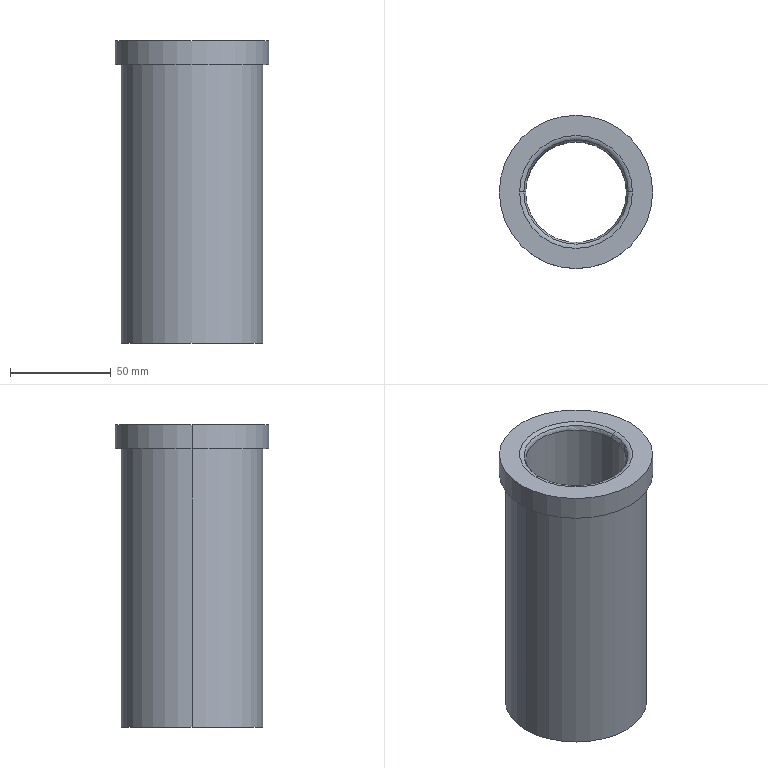Part | Creo | 1 solid | 17 faces | box 76 x 76 x 150 mm | volume 290376 mm3 | torus 8 | cylinder 6 | plane 3 | commonest cylinder face diameters 50 x2 70 x2 76 x2
STEP:
#1=CARTESIAN_POINT('',(-212.,297.,0.5));
#2=VERTEX_POINT('',#1);
#3=CARTESIAN_POINT('',(-282.,297.,0.5));
#4=VERTEX_POINT('',#3);
#5=CARTESIAN_POINT('',(-247.,297.,0.5));
#6=DIRECTION('',(0.,0.,-1.));
#7=DIRECTION('',(1.,0.,0.));
#8=AXIS2_PLACEMENT_3D('',#5,#6,#7);
#9=CIRCLE('',#8,35.);
#10=EDGE_CURVE('',#2,#4,#9,.T.);
#11=ORIENTED_EDGE('',*,*,#10,.F.);
#12=CARTESIAN_POINT('',(-247.,297.,0.5));
#13=DIRECTION('',(0.,0.,-1.));
#14=DIRECTION('',(-1.,0.,0.));
#15=AXIS2_PLACEMENT_3D('',#12,#13,#14);
#16=CIRCLE('',#15,35.);
#17=EDGE_CURVE('',#4,#2,#16,.T.);
#18=ORIENTED_EDGE('',*,*,#17,.F.);
#19=EDGE_LOOP('',(#11,#18));
#20=FACE_OUTER_BOUND('',#19,.F.);
#21=CARTESIAN_POINT('',(-275.,297.,0.5));
#22=VERTEX_POINT('',#21);
#23=CARTESIAN_POINT('',(-219.,297.,0.5));
#24=VERTEX_POINT('',#23);
#25=CARTESIAN_POINT('',(-247.,297.,0.5));
#26=DIRECTION('',(0.,0.,1.));
#27=DIRECTION('',(-1.,0.,0.));
#28=AXIS2_PLACEMENT_3D('',#25,#26,#27);
#29=CIRCLE('',#28,28.);
#30=EDGE_CURVE('',#22,#24,#29,.T.);
#31=ORIENTED_EDGE('',*,*,#30,.F.);
#32=CARTESIAN_POINT('',(-247.,297.,0.5));
#33=DIRECTION('',(0.,0.,1.));
#34=DIRECTION('',(1.,0.,0.));
#35=AXIS2_PLACEMENT_3D('',#32,#33,#34);
#36=CIRCLE('',#35,28.);
#37=EDGE_CURVE('',#24,#22,#36,.T.);
#38=ORIENTED_EDGE('',*,*,#37,.F.);
#39=EDGE_LOOP('',(#31,#38));
#40=FACE_BOUND('',#39,.F.);
#41=CARTESIAN_POINT('',(-247.,297.,0.5));
#42=DIRECTION('',(0.,0.,-1.));
#43=DIRECTION('',(-1.,0.,0.));
#44=AXIS2_PLACEMENT_3D('',#41,#42,#43);
#45=PLANE('',#44);
#46=ADVANCED_FACE('',(#20,#40),#45,.T.);
#47=ORIENTED_EDGE('',*,*,#30,.T.);
#48=CARTESIAN_POINT('',(-221.121,297.,1.379));
#49=VERTEX_POINT('',#48);
#50=CARTESIAN_POINT('',(-219.,297.,3.5));
#51=DIRECTION('',(0.,1.,0.));
#52=DIRECTION('',(0.,0.,-1.));
#53=AXIS2_PLACEMENT_3D('',#50,#51,#52);
#54=CIRCLE('',#53,3.);
#55=EDGE_CURVE('',#24,#49,#54,.T.);
#56=ORIENTED_EDGE('',*,*,#55,.T.);
#57=CARTESIAN_POINT('',(-272.879,297.,1.379));
#58=VERTEX_POINT('',#57);
#59=CARTESIAN_POINT('',(-247.,297.,1.379));
#60=DIRECTION('',(0.,0.,-1.));
#61=DIRECTION('',(1.,0.,0.));
#62=AXIS2_PLACEMENT_3D('',#59,#60,#61);
#63=CIRCLE('',#62,25.879);
#64=EDGE_CURVE('',#49,#58,#63,.T.);
#65=ORIENTED_EDGE('',*,*,#64,.T.);
#66=CARTESIAN_POINT('',(-275.,297.,3.5));
#67=DIRECTION('',(0.,-1.,0.));
#68=DIRECTION('',(0.,0.,-1.));
#69=AXIS2_PLACEMENT_3D('',#66,#67,#68);
#70=CIRCLE('',#69,3.);
#71=EDGE_CURVE('',#22,#58,#70,.T.);
#72=ORIENTED_EDGE('',*,*,#71,.F.);
#73=EDGE_LOOP('',(#47,#56,#65,#72));
#74=FACE_OUTER_BOUND('',#73,.F.);
#75=CARTESIAN_POINT('',(-247.,297.,3.5));
#76=DIRECTION('',(0.,0.,-1.));
#77=DIRECTION('',(-1.,0.,0.));
#78=AXIS2_PLACEMENT_3D('',#75,#76,#77);
#79=TOROIDAL_SURFACE('',#78,28.,3.);
#80=ADVANCED_FACE('',(#74),#79,.T.);
#81=ORIENTED_EDGE('',*,*,#37,.T.);
#82=ORIENTED_EDGE('',*,*,#71,.T.);
#83=CARTESIAN_POINT('',(-247.,297.,1.379));
#84=DIRECTION('',(0.,0.,-1.));
#85=DIRECTION('',(-1.,0.,0.));
#86=AXIS2_PLACEMENT_3D('',#83,#84,#85);
#87=CIRCLE('',#86,25.879);
#88=EDGE_CURVE('',#58,#49,#87,.T.);
#89=ORIENTED_EDGE('',*,*,#88,.T.);
#90=ORIENTED_EDGE('',*,*,#55,.F.);
#91=EDGE_LOOP('',(#81,#82,#89,#90));
#92=FACE_OUTER_BOUND('',#91,.F.);
#93=CARTESIAN_POINT('',(-247.,297.,3.5));
#94=DIRECTION('',(0.,0.,-1.));
#95=DIRECTION('',(-1.,0.,0.));
#96=AXIS2_PLACEMENT_3D('',#93,#94,#95);
#97=TOROIDAL_SURFACE('',#96,28.,3.);
#98=ADVANCED_FACE('',(#92),#97,.T.);
#99=CARTESIAN_POINT('',(-222.,297.,3.5));
#100=VERTEX_POINT('',#99);
#101=CARTESIAN_POINT('',(-272.,297.,3.5));
#102=VERTEX_POINT('',#101);
#103=CARTESIAN_POINT('',(-247.,297.,3.5));
#104=DIRECTION('',(0.,0.,1.));
#105=DIRECTION('',(1.,0.,0.));
#106=AXIS2_PLACEMENT_3D('',#103,#104,#105);
#107=CIRCLE('',#106,25.);
#108=EDGE_CURVE('',#100,#102,#107,.T.);
#109=ORIENTED_EDGE('',*,*,#108,.F.);
#110=CARTESIAN_POINT('',(-219.,297.,3.5));
#111=DIRECTION('',(0.,1.,0.));
#112=DIRECTION('',(-0.7071,0.,-0.7071));
#113=AXIS2_PLACEMENT_3D('',#110,#111,#112);
#114=CIRCLE('',#113,3.);
#115=EDGE_CURVE('',#49,#100,#114,.T.);
#116=ORIENTED_EDGE('',*,*,#115,.F.);
#117=ORIENTED_EDGE('',*,*,#88,.F.);
#118=CARTESIAN_POINT('',(-275.,297.,3.5));
#119=DIRECTION('',(0.,-1.,0.));
#120=DIRECTION('',(0.7071,0.,-0.7071));
#121=AXIS2_PLACEMENT_3D('',#118,#119,#120);
#122=CIRCLE('',#121,3.);
#123=EDGE_CURVE('',#58,#102,#122,.T.);
#124=ORIENTED_EDGE('',*,*,#123,.T.);
#125=EDGE_LOOP('',(#109,#116,#117,#124));
#126=FACE_OUTER_BOUND('',#125,.F.);
#127=CARTESIAN_POINT('',(-247.,297.,3.5));
#128=DIRECTION('',(0.,0.,-1.));
#129=DIRECTION('',(-1.,0.,0.));
#130=AXIS2_PLACEMENT_3D('',#127,#128,#129);
#131=TOROIDAL_SURFACE('',#130,28.,3.);
#132=ADVANCED_FACE('',(#126),#131,.T.);
#133=CARTESIAN_POINT('',(-272.,297.,147.5));
#134=VERTEX_POINT('',#133);
#135=CARTESIAN_POINT('',(-222.,297.,147.5));
#136=VERTEX_POINT('',#135);
#137=CARTESIAN_POINT('',(-247.,297.,147.5));
#138=DIRECTION('',(0.,0.,-1.));
#139=DIRECTION('',(-1.,0.,0.));
#140=AXIS2_PLACEMENT_3D('',#137,#138,#139);
#141=CIRCLE('',#140,25.);
#142=EDGE_CURVE('',#134,#136,#141,.T.);
#143=ORIENTED_EDGE('',*,*,#142,.T.);
#144=CARTESIAN_POINT('',(-222.,297.,147.5));
#145=DIRECTION('',(0.,0.,-1.));
#146=VECTOR('',#145,144.);
#147=LINE('',#144,#146);
#148=EDGE_CURVE('',#136,#100,#147,.T.);
#149=ORIENTED_EDGE('',*,*,#148,.T.);
#150=ORIENTED_EDGE('',*,*,#108,.T.);
#151=CARTESIAN_POINT('',(-272.,297.,147.5));
#152=DIRECTION('',(0.,0.,-1.));
#153=VECTOR('',#152,144.);
#154=LINE('',#151,#153);
#155=EDGE_CURVE('',#134,#102,#154,.T.);
#156=ORIENTED_EDGE('',*,*,#155,.F.);
#157=EDGE_LOOP('',(#143,#149,#150,#156));
#158=FACE_OUTER_BOUND('',#157,.F.);
#159=CARTESIAN_POINT('',(-247.,297.,220.5));
#160=DIRECTION('',(0.,0.,-1.));
#161=DIRECTION('',(-1.,0.,0.));
#162=AXIS2_PLACEMENT_3D('',#159,#160,#161);
#163=CYLINDRICAL_SURFACE('',#162,25.);
#164=ADVANCED_FACE('',(#158),#163,.F.);
#165=ORIENTED_EDGE('',*,*,#142,.F.);
#166=CARTESIAN_POINT('',(-272.879,297.,149.621));
#167=VERTEX_POINT('',#166);
#168=CARTESIAN_POINT('',(-275.,297.,147.5));
#169=DIRECTION('',(0.,1.,0.));
#170=DIRECTION('',(0.7071,0.,0.7071));
#171=AXIS2_PLACEMENT_3D('',#168,#169,#170);
#172=CIRCLE('',#171,3.);
#173=EDGE_CURVE('',#167,#134,#172,.T.);
#174=ORIENTED_EDGE('',*,*,#173,.F.);
#175=CARTESIAN_POINT('',(-221.121,297.,149.621));
#176=VERTEX_POINT('',#175);
#177=CARTESIAN_POINT('',(-247.,297.,149.621));
#178=DIRECTION('',(0.,0.,1.));
#179=DIRECTION('',(1.,0.,0.));
#180=AXIS2_PLACEMENT_3D('',#177,#178,#179);
#181=CIRCLE('',#180,25.879);
#182=EDGE_CURVE('',#176,#167,#181,.T.);
#183=ORIENTED_EDGE('',*,*,#182,.F.);
#184=CARTESIAN_POINT('',(-219.,297.,147.5));
#185=DIRECTION('',(0.,-1.,0.));
#186=DIRECTION('',(-0.7071,0.,0.7071));
#187=AXIS2_PLACEMENT_3D('',#184,#185,#186);
#188=CIRCLE('',#187,3.);
#189=EDGE_CURVE('',#176,#136,#188,.T.);
#190=ORIENTED_EDGE('',*,*,#189,.T.);
#191=EDGE_LOOP('',(#165,#174,#183,#190));
#192=FACE_OUTER_BOUND('',#191,.F.);
#193=CARTESIAN_POINT('',(-247.,297.,147.5));
#194=DIRECTION('',(0.,0.,1.));
#195=DIRECTION('',(1.,0.,0.));
#196=AXIS2_PLACEMENT_3D('',#193,#194,#195);
#197=TOROIDAL_SURFACE('',#196,28.,3.);
#198=ADVANCED_FACE('',(#192),#197,.T.);
#199=CARTESIAN_POINT('',(-247.,297.,147.5));
#200=DIRECTION('',(0.,0.,-1.));
#201=DIRECTION('',(1.,0.,0.));
#202=AXIS2_PLACEMENT_3D('',#199,#200,#201);
#203=CIRCLE('',#202,25.);
#204=EDGE_CURVE('',#136,#134,#203,.T.);
#205=ORIENTED_EDGE('',*,*,#204,.F.);
#206=ORIENTED_EDGE('',*,*,#189,.F.);
#207=CARTESIAN_POINT('',(-247.,297.,149.621));
#208=DIRECTION('',(0.,0.,1.));
#209=DIRECTION('',(-1.,0.,0.));
#210=AXIS2_PLACEMENT_3D('',#207,#208,#209);
#211=CIRCLE('',#210,25.879);
#212=EDGE_CURVE('',#167,#176,#211,.T.);
#213=ORIENTED_EDGE('',*,*,#212,.F.);
#214=ORIENTED_EDGE('',*,*,#173,.T.);
#215=EDGE_LOOP('',(#205,#206,#213,#214));
#216=FACE_OUTER_BOUND('',#215,.F.);
#217=CARTESIAN_POINT('',(-247.,297.,147.5));
#218=DIRECTION('',(0.,0.,1.));
#219=DIRECTION('',(1.,0.,0.));
#220=AXIS2_PLACEMENT_3D('',#217,#218,#219);
#221=TOROIDAL_SURFACE('',#220,28.,3.);
#222=ADVANCED_FACE('',(#216),#221,.T.);
#223=ORIENTED_EDGE('',*,*,#204,.T.);
#224=ORIENTED_EDGE('',*,*,#155,.T.);
#225=CARTESIAN_POINT('',(-247.,297.,3.5));
#226=DIRECTION('',(0.,0.,1.));
#227=DIRECTION('',(-1.,0.,0.));
#228=AXIS2_PLACEMENT_3D('',#225,#226,#227);
#229=CIRCLE('',#228,25.);
#230=EDGE_CURVE('',#102,#100,#229,.T.);
#231=ORIENTED_EDGE('',*,*,#230,.T.);
#232=ORIENTED_EDGE('',*,*,#148,.F.);
#233=EDGE_LOOP('',(#223,#224,#231,#232));
#234=FACE_OUTER_BOUND('',#233,.F.);
#235=CARTESIAN_POINT('',(-247.,297.,220.5));
#236=DIRECTION('',(0.,0.,-1.));
#237=DIRECTION('',(-1.,0.,0.));
#238=AXIS2_PLACEMENT_3D('',#235,#236,#237);
#239=CYLINDRICAL_SURFACE('',#238,25.);
#240=ADVANCED_FACE('',(#234),#239,.F.);
#241=ORIENTED_EDGE('',*,*,#230,.F.);
#242=ORIENTED_EDGE('',*,*,#123,.F.);
#243=ORIENTED_EDGE('',*,*,#64,.F.);
#244=ORIENTED_EDGE('',*,*,#115,.T.);
#245=EDGE_LOOP('',(#241,#242,#243,#244));
#246=FACE_OUTER_BOUND('',#245,.F.);
#247=CARTESIAN_POINT('',(-247.,297.,3.5));
#248=DIRECTION('',(0.,0.,-1.));
#249=DIRECTION('',(-1.,0.,0.));
#250=AXIS2_PLACEMENT_3D('',#247,#248,#249);
#251=TOROIDAL_SURFACE('',#250,28.,3.);
#252=ADVANCED_FACE('',(#246),#251,.T.);
#253=CARTESIAN_POINT('',(-219.,297.,150.5));
#254=VERTEX_POINT('',#253);
#255=CARTESIAN_POINT('',(-275.,297.,150.5));
#256=VERTEX_POINT('',#255);
#257=CARTESIAN_POINT('',(-247.,297.,150.5));
#258=DIRECTION('',(0.,0.,-1.));
#259=DIRECTION('',(1.,0.,0.));
#260=AXIS2_PLACEMENT_3D('',#257,#258,#259);
#261=CIRCLE('',#260,28.);
#262=EDGE_CURVE('',#254,#256,#261,.T.);
#263=ORIENTED_EDGE('',*,*,#262,.T.);
#264=CARTESIAN_POINT('',(-275.,297.,147.5));
#265=DIRECTION('',(0.,1.,0.));
#266=DIRECTION('',(0.,0.,1.));
#267=AXIS2_PLACEMENT_3D('',#264,#265,#266);
#268=CIRCLE('',#267,3.);
#269=EDGE_CURVE('',#256,#167,#268,.T.);
#270=ORIENTED_EDGE('',*,*,#269,.T.);
#271=ORIENTED_EDGE('',*,*,#212,.T.);
#272=CARTESIAN_POINT('',(-219.,297.,147.5));
#273=DIRECTION('',(0.,-1.,0.));
#274=DIRECTION('',(0.,0.,1.));
#275=AXIS2_PLACEMENT_3D('',#272,#273,#274);
#276=CIRCLE('',#275,3.);
#277=EDGE_CURVE('',#254,#176,#276,.T.);
#278=ORIENTED_EDGE('',*,*,#277,.F.);
#279=EDGE_LOOP('',(#263,#270,#271,#278));
#280=FACE_OUTER_BOUND('',#279,.F.);
#281=CARTESIAN_POINT('',(-247.,297.,147.5));
#282=DIRECTION('',(0.,0.,1.));
#283=DIRECTION('',(1.,0.,0.));
#284=AXIS2_PLACEMENT_3D('',#281,#282,#283);
#285=TOROIDAL_SURFACE('',#284,28.,3.);
#286=ADVANCED_FACE('',(#280),#285,.T.);
#287=CARTESIAN_POINT('',(-285.,297.,150.5));
#288=VERTEX_POINT('',#287);
#289=CARTESIAN_POINT('',(-209.,297.,150.5));
#290=VERTEX_POINT('',#289);
#291=CARTESIAN_POINT('',(-247.,297.,150.5));
#292=DIRECTION('',(0.,0.,1.));
#293=DIRECTION('',(-1.,0.,0.));
#294=AXIS2_PLACEMENT_3D('',#291,#292,#293);
#295=CIRCLE('',#294,38.);
#296=EDGE_CURVE('',#288,#290,#295,.T.);
#297=ORIENTED_EDGE('',*,*,#296,.F.);
#298=CARTESIAN_POINT('',(-247.,297.,150.5));
#299=DIRECTION('',(0.,0.,1.));
#300=DIRECTION('',(1.,0.,0.));
#301=AXIS2_PLACEMENT_3D('',#298,#299,#300);
#302=CIRCLE('',#301,38.);
#303=EDGE_CURVE('',#290,#288,#302,.T.);
#304=ORIENTED_EDGE('',*,*,#303,.F.);
#305=EDGE_LOOP('',(#297,#304));
#306=FACE_OUTER_BOUND('',#305,.F.);
#307=ORIENTED_EDGE('',*,*,#262,.F.);
#308=CARTESIAN_POINT('',(-247.,297.,150.5));
#309=DIRECTION('',(0.,0.,-1.));
#310=DIRECTION('',(-1.,0.,0.));
#311=AXIS2_PLACEMENT_3D('',#308,#309,#310);
#312=CIRCLE('',#311,28.);
#313=EDGE_CURVE('',#256,#254,#312,.T.);
#314=ORIENTED_EDGE('',*,*,#313,.F.);
#315=EDGE_LOOP('',(#307,#314));
#316=FACE_BOUND('',#315,.F.);
#317=CARTESIAN_POINT('',(-247.,297.,150.5));
#318=DIRECTION('',(0.,0.,1.));
#319=DIRECTION('',(1.,0.,0.));
#320=AXIS2_PLACEMENT_3D('',#317,#318,#319);
#321=PLANE('',#320);
#322=ADVANCED_FACE('',(#306,#316),#321,.T.);
#323=ORIENTED_EDGE('',*,*,#313,.T.);
#324=ORIENTED_EDGE('',*,*,#277,.T.);
#325=ORIENTED_EDGE('',*,*,#182,.T.);
#326=ORIENTED_EDGE('',*,*,#269,.F.);
#327=EDGE_LOOP('',(#323,#324,#325,#326));
#328=FACE_OUTER_BOUND('',#327,.F.);
#329=CARTESIAN_POINT('',(-247.,297.,147.5));
#330=DIRECTION('',(0.,0.,1.));
#331=DIRECTION('',(1.,0.,0.));
#332=AXIS2_PLACEMENT_3D('',#329,#330,#331);
#333=TOROIDAL_SURFACE('',#332,28.,3.);
#334=ADVANCED_FACE('',(#328),#333,.T.);
#335=CARTESIAN_POINT('',(-209.,297.,138.5));
#336=VERTEX_POINT('',#335);
#337=CARTESIAN_POINT('',(-285.,297.,138.5));
#338=VERTEX_POINT('',#337);
#339=CARTESIAN_POINT('',(-247.,297.,138.5));
#340=DIRECTION('',(0.,0.,-1.));
#341=DIRECTION('',(1.,0.,0.));
#342=AXIS2_PLACEMENT_3D('',#339,#340,#341);
#343=CIRCLE('',#342,38.);
#344=EDGE_CURVE('',#336,#338,#343,.T.);
#345=ORIENTED_EDGE('',*,*,#344,.T.);
#346=CARTESIAN_POINT('',(-285.,297.,150.5));
#347=DIRECTION('',(0.,0.,-1.));
#348=VECTOR('',#347,12.);
#349=LINE('',#346,#348);
#350=EDGE_CURVE('',#288,#338,#349,.T.);
#351=ORIENTED_EDGE('',*,*,#350,.F.);
#352=ORIENTED_EDGE('',*,*,#296,.T.);
#353=CARTESIAN_POINT('',(-209.,297.,150.5));
#354=DIRECTION('',(0.,0.,-1.));
#355=VECTOR('',#354,12.);
#356=LINE('',#353,#355);
#357=EDGE_CURVE('',#290,#336,#356,.T.);
#358=ORIENTED_EDGE('',*,*,#357,.T.);
#359=EDGE_LOOP('',(#345,#351,#352,#358));
#360=FACE_OUTER_BOUND('',#359,.F.);
#361=CARTESIAN_POINT('',(-247.,297.,150.5));
#362=DIRECTION('',(0.,0.,-1.));
#363=DIRECTION('',(-1.,0.,0.));
#364=AXIS2_PLACEMENT_3D('',#361,#362,#363);
#365=CYLINDRICAL_SURFACE('',#364,38.);
#366=ADVANCED_FACE('',(#360),#365,.T.);
#367=ORIENTED_EDGE('',*,*,#344,.F.);
#368=CARTESIAN_POINT('',(-247.,297.,138.5));
#369=DIRECTION('',(0.,0.,-1.));
#370=DIRECTION('',(-1.,0.,0.));
#371=AXIS2_PLACEMENT_3D('',#368,#369,#370);
#372=CIRCLE('',#371,38.);
#373=EDGE_CURVE('',#338,#336,#372,.T.);
#374=ORIENTED_EDGE('',*,*,#373,.F.);
#375=EDGE_LOOP('',(#367,#374));
#376=FACE_OUTER_BOUND('',#375,.F.);
#377=CARTESIAN_POINT('',(-282.,297.,138.5));
#378=VERTEX_POINT('',#377);
#379=CARTESIAN_POINT('',(-212.,297.,138.5));
#380=VERTEX_POINT('',#379);
#381=CARTESIAN_POINT('',(-247.,297.,138.5));
#382=DIRECTION('',(0.,0.,1.));
#383=DIRECTION('',(-1.,0.,0.));
#384=AXIS2_PLACEMENT_3D('',#381,#382,#383);
#385=CIRCLE('',#384,35.);
#386=EDGE_CURVE('',#378,#380,#385,.T.);
#387=ORIENTED_EDGE('',*,*,#386,.F.);
#388=CARTESIAN_POINT('',(-247.,297.,138.5));
#389=DIRECTION('',(0.,0.,1.));
#390=DIRECTION('',(1.,0.,0.));
#391=AXIS2_PLACEMENT_3D('',#388,#389,#390);
#392=CIRCLE('',#391,35.);
#393=EDGE_CURVE('',#380,#378,#392,.T.);
#394=ORIENTED_EDGE('',*,*,#393,.F.);
#395=EDGE_LOOP('',(#387,#394));
#396=FACE_BOUND('',#395,.F.);
#397=CARTESIAN_POINT('',(-247.,297.,138.5));
#398=DIRECTION('',(0.,0.,-1.));
#399=DIRECTION('',(-1.,0.,0.));
#400=AXIS2_PLACEMENT_3D('',#397,#398,#399);
#401=PLANE('',#400);
#402=ADVANCED_FACE('',(#376,#396),#401,.T.);
#403=ORIENTED_EDGE('',*,*,#386,.T.);
#404=CARTESIAN_POINT('',(-212.,297.,138.5));
#405=DIRECTION('',(0.,0.,-1.));
#406=VECTOR('',#405,138.);
#407=LINE('',#404,#406);
#408=EDGE_CURVE('',#380,#2,#407,.T.);
#409=ORIENTED_EDGE('',*,*,#408,.T.);
#410=ORIENTED_EDGE('',*,*,#10,.T.);
#411=CARTESIAN_POINT('',(-282.,297.,138.5));
#412=DIRECTION('',(0.,0.,-1.));
#413=VECTOR('',#412,138.);
#414=LINE('',#411,#413);
#415=EDGE_CURVE('',#378,#4,#414,.T.);
#416=ORIENTED_EDGE('',*,*,#415,.F.);
#417=EDGE_LOOP('',(#403,#409,#410,#416));
#418=FACE_OUTER_BOUND('',#417,.F.);
#419=CARTESIAN_POINT('',(-247.,297.,220.5));
#420=DIRECTION('',(0.,0.,-1.));
#421=DIRECTION('',(-1.,0.,0.));
#422=AXIS2_PLACEMENT_3D('',#419,#420,#421);
#423=CYLINDRICAL_SURFACE('',#422,35.);
#424=ADVANCED_FACE('',(#418),#423,.T.);
#425=ORIENTED_EDGE('',*,*,#393,.T.);
#426=ORIENTED_EDGE('',*,*,#415,.T.);
#427=ORIENTED_EDGE('',*,*,#17,.T.);
#428=ORIENTED_EDGE('',*,*,#408,.F.);
#429=EDGE_LOOP('',(#425,#426,#427,#428));
#430=FACE_OUTER_BOUND('',#429,.F.);
#431=CARTESIAN_POINT('',(-247.,297.,220.5));
#432=DIRECTION('',(0.,0.,-1.));
#433=DIRECTION('',(-1.,0.,0.));
#434=AXIS2_PLACEMENT_3D('',#431,#432,#433);
#435=CYLINDRICAL_SURFACE('',#434,35.);
#436=ADVANCED_FACE('',(#430),#435,.T.);
#437=ORIENTED_EDGE('',*,*,#373,.T.);
#438=ORIENTED_EDGE('',*,*,#357,.F.);
#439=ORIENTED_EDGE('',*,*,#303,.T.);
#440=ORIENTED_EDGE('',*,*,#350,.T.);
#441=EDGE_LOOP('',(#437,#438,#439,#440));
#442=FACE_OUTER_BOUND('',#441,.F.);
#443=CARTESIAN_POINT('',(-247.,297.,150.5));
#444=DIRECTION('',(0.,0.,-1.));
#445=DIRECTION('',(-1.,0.,0.));
#446=AXIS2_PLACEMENT_3D('',#443,#444,#445);
#447=CYLINDRICAL_SURFACE('',#446,38.);
#448=ADVANCED_FACE('',(#442),#447,.T.);
#449=CLOSED_SHELL('',(#46,#80,#98,#132,#164,#198,#222,#240,#252,#286,#322,#334,#366,#402,#424,#436,#448));
#450=MANIFOLD_SOLID_BREP('',#449);
#451=(LENGTH_UNIT()NAMED_UNIT(*)SI_UNIT(.MILLI.,.METRE.));
#452=UNCERTAINTY_MEASURE_WITH_UNIT(LENGTH_MEASURE(0.01845),#451,'','');
#453=(NAMED_UNIT(*)PLANE_ANGLE_UNIT()SI_UNIT($,.RADIAN.));
#454=PLANE_ANGLE_MEASURE_WITH_UNIT(PLANE_ANGLE_MEASURE(0.01745),#453);
#455=(CONVERSION_BASED_UNIT('DEGREE',#454)NAMED_UNIT(*)PLANE_ANGLE_UNIT());
#456=(NAMED_UNIT(*)SI_UNIT($,.STERADIAN.)SOLID_ANGLE_UNIT());
#457=(GEOMETRIC_REPRESENTATION_CONTEXT(3)GLOBAL_UNCERTAINTY_ASSIGNED_CONTEXT((#452))GLOBAL_UNIT_ASSIGNED_CONTEXT((#451,#455,#456))REPRESENTATION_CONTEXT('',''));
#458=ADVANCED_BREP_SHAPE_REPRESENTATION('',(#450),#457);